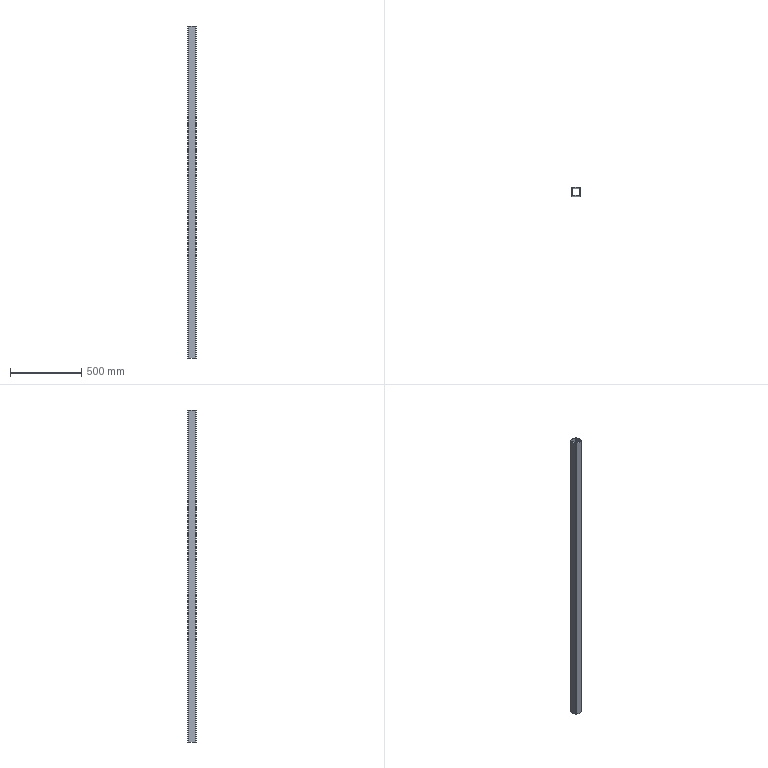Part | STEP file | 750038153 | 1 solid | 18 faces | box 60 x 60 x 2327 mm | volume 2020637 mm3 | plane 10 | cylinder 8 | commonest cylinder face diameters 4 x4 12 x4
STEP:
#1=CARTESIAN_POINT('',(-26.,24.,2326.5));
#2=VERTEX_POINT('',#1);
#3=CARTESIAN_POINT('',(-26.,24.,0.));
#4=VERTEX_POINT('',#3);
#5=CARTESIAN_POINT('',(-26.,24.,2326.5));
#6=DIRECTION('',(0.,0.,-1.));
#7=VECTOR('',#6,1000.);
#8=LINE('',#5,#7);
#9=EDGE_CURVE('',#2,#4,#8,.T.);
#10=ORIENTED_EDGE('',*,*,#9,.F.);
#11=CARTESIAN_POINT('',(-26.,-24.,2326.5));
#12=VERTEX_POINT('',#11);
#13=CARTESIAN_POINT('',(-26.,-24.,2326.5));
#14=DIRECTION('',(0.,1.,0.));
#15=VECTOR('',#14,1000.);
#16=LINE('',#13,#15);
#17=EDGE_CURVE('',#12,#2,#16,.T.);
#18=ORIENTED_EDGE('',*,*,#17,.F.);
#19=CARTESIAN_POINT('',(-26.,-24.,0.));
#20=VERTEX_POINT('',#19);
#21=CARTESIAN_POINT('',(-26.,-24.,2326.5));
#22=DIRECTION('',(0.,0.,1.));
#23=VECTOR('',#22,1000.);
#24=LINE('',#21,#23);
#25=EDGE_CURVE('',#20,#12,#24,.T.);
#26=ORIENTED_EDGE('',*,*,#25,.F.);
#27=CARTESIAN_POINT('',(-26.,-24.,0.));
#28=DIRECTION('',(0.,-1.,0.));
#29=VECTOR('',#28,1000.);
#30=LINE('',#27,#29);
#31=EDGE_CURVE('',#4,#20,#30,.T.);
#32=ORIENTED_EDGE('',*,*,#31,.F.);
#33=EDGE_LOOP('',(#10,#18,#26,#32));
#34=FACE_OUTER_BOUND('',#33,.T.);
#35=CARTESIAN_POINT('',(-26.,-24.,2326.5));
#36=DIRECTION('',(-1.,0.,0.));
#37=DIRECTION('',(0.,-1.,0.));
#38=AXIS2_PLACEMENT_3D('',#35,#36,#37);
#39=PLANE('',#38);
#40=ADVANCED_FACE('',(#34),#39,.F.);
#41=CARTESIAN_POINT('',(26.,24.,0.));
#42=VERTEX_POINT('',#41);
#43=CARTESIAN_POINT('',(24.,26.,0.));
#44=VERTEX_POINT('',#43);
#45=CARTESIAN_POINT('',(24.,24.,0.));
#46=DIRECTION('',(0.,0.,1.));
#47=DIRECTION('',(-1.,0.,0.));
#48=AXIS2_PLACEMENT_3D('',#45,#46,#47);
#49=CIRCLE('',#48,2.);
#50=EDGE_CURVE('',#42,#44,#49,.T.);
#51=ORIENTED_EDGE('',*,*,#50,.T.);
#52=CARTESIAN_POINT('',(-24.,26.,0.));
#53=VERTEX_POINT('',#52);
#54=CARTESIAN_POINT('',(24.,26.,0.));
#55=DIRECTION('',(-1.,0.,0.));
#56=VECTOR('',#55,1000.);
#57=LINE('',#54,#56);
#58=EDGE_CURVE('',#44,#53,#57,.T.);
#59=ORIENTED_EDGE('',*,*,#58,.T.);
#60=CARTESIAN_POINT('',(-24.,24.,0.));
#61=DIRECTION('',(0.,0.,1.));
#62=DIRECTION('',(-1.,0.,0.));
#63=AXIS2_PLACEMENT_3D('',#60,#61,#62);
#64=CIRCLE('',#63,2.);
#65=EDGE_CURVE('',#53,#4,#64,.T.);
#66=ORIENTED_EDGE('',*,*,#65,.T.);
#67=ORIENTED_EDGE('',*,*,#31,.T.);
#68=CARTESIAN_POINT('',(-24.,-26.,0.));
#69=VERTEX_POINT('',#68);
#70=CARTESIAN_POINT('',(-24.,-24.,0.));
#71=DIRECTION('',(0.,0.,1.));
#72=DIRECTION('',(-1.,0.,0.));
#73=AXIS2_PLACEMENT_3D('',#70,#71,#72);
#74=CIRCLE('',#73,2.);
#75=EDGE_CURVE('',#20,#69,#74,.T.);
#76=ORIENTED_EDGE('',*,*,#75,.T.);
#77=CARTESIAN_POINT('',(24.,-26.,0.));
#78=VERTEX_POINT('',#77);
#79=CARTESIAN_POINT('',(24.,-26.,0.));
#80=DIRECTION('',(1.,0.,0.));
#81=VECTOR('',#80,1000.);
#82=LINE('',#79,#81);
#83=EDGE_CURVE('',#69,#78,#82,.T.);
#84=ORIENTED_EDGE('',*,*,#83,.T.);
#85=CARTESIAN_POINT('',(26.,-24.,0.));
#86=VERTEX_POINT('',#85);
#87=CARTESIAN_POINT('',(24.,-24.,0.));
#88=DIRECTION('',(0.,0.,1.));
#89=DIRECTION('',(-1.,0.,0.));
#90=AXIS2_PLACEMENT_3D('',#87,#88,#89);
#91=CIRCLE('',#90,2.);
#92=EDGE_CURVE('',#78,#86,#91,.T.);
#93=ORIENTED_EDGE('',*,*,#92,.T.);
#94=CARTESIAN_POINT('',(26.,-24.,0.));
#95=DIRECTION('',(0.,1.,0.));
#96=VECTOR('',#95,1000.);
#97=LINE('',#94,#96);
#98=EDGE_CURVE('',#86,#42,#97,.T.);
#99=ORIENTED_EDGE('',*,*,#98,.T.);
#100=EDGE_LOOP('',(#51,#59,#66,#67,#76,#84,#93,#99));
#101=FACE_BOUND('',#100,.T.);
#102=CARTESIAN_POINT('',(-24.,30.,0.));
#103=VERTEX_POINT('',#102);
#104=CARTESIAN_POINT('',(24.,30.,0.));
#105=VERTEX_POINT('',#104);
#106=CARTESIAN_POINT('',(24.,30.,0.));
#107=DIRECTION('',(1.,0.,0.));
#108=VECTOR('',#107,1000.);
#109=LINE('',#106,#108);
#110=EDGE_CURVE('',#103,#105,#109,.T.);
#111=ORIENTED_EDGE('',*,*,#110,.T.);
#112=CARTESIAN_POINT('',(30.,24.,0.));
#113=VERTEX_POINT('',#112);
#114=CARTESIAN_POINT('',(24.,24.,0.));
#115=DIRECTION('',(0.,0.,-1.));
#116=DIRECTION('',(-1.,0.,0.));
#117=AXIS2_PLACEMENT_3D('',#114,#115,#116);
#118=CIRCLE('',#117,6.);
#119=EDGE_CURVE('',#105,#113,#118,.T.);
#120=ORIENTED_EDGE('',*,*,#119,.T.);
#121=CARTESIAN_POINT('',(30.,-24.,0.));
#122=VERTEX_POINT('',#121);
#123=CARTESIAN_POINT('',(30.,-24.,0.));
#124=DIRECTION('',(0.,-1.,0.));
#125=VECTOR('',#124,1000.);
#126=LINE('',#123,#125);
#127=EDGE_CURVE('',#113,#122,#126,.T.);
#128=ORIENTED_EDGE('',*,*,#127,.T.);
#129=CARTESIAN_POINT('',(24.,-30.,0.));
#130=VERTEX_POINT('',#129);
#131=CARTESIAN_POINT('',(24.,-24.,0.));
#132=DIRECTION('',(0.,0.,-1.));
#133=DIRECTION('',(-1.,0.,0.));
#134=AXIS2_PLACEMENT_3D('',#131,#132,#133);
#135=CIRCLE('',#134,6.);
#136=EDGE_CURVE('',#122,#130,#135,.T.);
#137=ORIENTED_EDGE('',*,*,#136,.T.);
#138=CARTESIAN_POINT('',(-24.,-30.,0.));
#139=VERTEX_POINT('',#138);
#140=CARTESIAN_POINT('',(24.,-30.,0.));
#141=DIRECTION('',(-1.,0.,0.));
#142=VECTOR('',#141,1000.);
#143=LINE('',#140,#142);
#144=EDGE_CURVE('',#130,#139,#143,.T.);
#145=ORIENTED_EDGE('',*,*,#144,.T.);
#146=CARTESIAN_POINT('',(-30.,-24.,0.));
#147=VERTEX_POINT('',#146);
#148=CARTESIAN_POINT('',(-24.,-24.,0.));
#149=DIRECTION('',(0.,0.,-1.));
#150=DIRECTION('',(-1.,0.,0.));
#151=AXIS2_PLACEMENT_3D('',#148,#149,#150);
#152=CIRCLE('',#151,6.);
#153=EDGE_CURVE('',#139,#147,#152,.T.);
#154=ORIENTED_EDGE('',*,*,#153,.T.);
#155=CARTESIAN_POINT('',(-30.,24.,0.));
#156=VERTEX_POINT('',#155);
#157=CARTESIAN_POINT('',(-30.,-24.,0.));
#158=DIRECTION('',(0.,1.,0.));
#159=VECTOR('',#158,1000.);
#160=LINE('',#157,#159);
#161=EDGE_CURVE('',#147,#156,#160,.T.);
#162=ORIENTED_EDGE('',*,*,#161,.T.);
#163=CARTESIAN_POINT('',(-24.,24.,0.));
#164=DIRECTION('',(0.,0.,-1.));
#165=DIRECTION('',(-1.,0.,0.));
#166=AXIS2_PLACEMENT_3D('',#163,#164,#165);
#167=CIRCLE('',#166,6.);
#168=EDGE_CURVE('',#156,#103,#167,.T.);
#169=ORIENTED_EDGE('',*,*,#168,.T.);
#170=EDGE_LOOP('',(#111,#120,#128,#137,#145,#154,#162,#169));
#171=FACE_OUTER_BOUND('',#170,.T.);
#172=CARTESIAN_POINT('',(24.,-24.,0.));
#173=DIRECTION('',(0.,0.,-1.));
#174=DIRECTION('',(-1.,0.,0.));
#175=AXIS2_PLACEMENT_3D('',#172,#173,#174);
#176=PLANE('',#175);
#177=ADVANCED_FACE('',(#101,#171),#176,.T.);
#178=CARTESIAN_POINT('',(-24.,26.,2326.5));
#179=VERTEX_POINT('',#178);
#180=CARTESIAN_POINT('',(-24.,26.,2326.5));
#181=DIRECTION('',(0.,0.,-1.));
#182=VECTOR('',#181,1000.);
#183=LINE('',#180,#182);
#184=EDGE_CURVE('',#179,#53,#183,.T.);
#185=ORIENTED_EDGE('',*,*,#184,.F.);
#186=CARTESIAN_POINT('',(-24.,24.,2326.5));
#187=DIRECTION('',(0.,0.,-1.));
#188=DIRECTION('',(-1.,0.,0.));
#189=AXIS2_PLACEMENT_3D('',#186,#187,#188);
#190=CIRCLE('',#189,2.);
#191=EDGE_CURVE('',#2,#179,#190,.T.);
#192=ORIENTED_EDGE('',*,*,#191,.F.);
#193=ORIENTED_EDGE('',*,*,#9,.T.);
#194=ORIENTED_EDGE('',*,*,#65,.F.);
#195=EDGE_LOOP('',(#185,#192,#193,#194));
#196=FACE_OUTER_BOUND('',#195,.T.);
#197=CARTESIAN_POINT('',(-24.,24.,2326.5));
#198=DIRECTION('',(0.,0.,-1.));
#199=DIRECTION('',(-1.,0.,0.));
#200=AXIS2_PLACEMENT_3D('',#197,#198,#199);
#201=CYLINDRICAL_SURFACE('',#200,2.);
#202=ADVANCED_FACE('',(#196),#201,.F.);
#203=CARTESIAN_POINT('',(24.,26.,2326.5));
#204=VERTEX_POINT('',#203);
#205=CARTESIAN_POINT('',(24.,26.,2326.5));
#206=DIRECTION('',(-1.,0.,0.));
#207=VECTOR('',#206,1000.);
#208=LINE('',#205,#207);
#209=EDGE_CURVE('',#204,#179,#208,.T.);
#210=ORIENTED_EDGE('',*,*,#209,.F.);
#211=CARTESIAN_POINT('',(26.,24.,2326.5));
#212=VERTEX_POINT('',#211);
#213=CARTESIAN_POINT('',(24.,24.,2326.5));
#214=DIRECTION('',(0.,0.,1.));
#215=DIRECTION('',(-1.,0.,0.));
#216=AXIS2_PLACEMENT_3D('',#213,#214,#215);
#217=CIRCLE('',#216,2.);
#218=EDGE_CURVE('',#212,#204,#217,.T.);
#219=ORIENTED_EDGE('',*,*,#218,.F.);
#220=CARTESIAN_POINT('',(26.,-24.,2326.5));
#221=VERTEX_POINT('',#220);
#222=CARTESIAN_POINT('',(26.,-24.,2326.5));
#223=DIRECTION('',(0.,1.,0.));
#224=VECTOR('',#223,1000.);
#225=LINE('',#222,#224);
#226=EDGE_CURVE('',#221,#212,#225,.T.);
#227=ORIENTED_EDGE('',*,*,#226,.F.);
#228=CARTESIAN_POINT('',(24.,-26.,2326.5));
#229=VERTEX_POINT('',#228);
#230=CARTESIAN_POINT('',(24.,-24.,2326.5));
#231=DIRECTION('',(0.,0.,1.));
#232=DIRECTION('',(-1.,0.,0.));
#233=AXIS2_PLACEMENT_3D('',#230,#231,#232);
#234=CIRCLE('',#233,2.);
#235=EDGE_CURVE('',#229,#221,#234,.T.);
#236=ORIENTED_EDGE('',*,*,#235,.F.);
#237=CARTESIAN_POINT('',(-24.,-26.,2326.5));
#238=VERTEX_POINT('',#237);
#239=CARTESIAN_POINT('',(24.,-26.,2326.5));
#240=DIRECTION('',(1.,0.,0.));
#241=VECTOR('',#240,1000.);
#242=LINE('',#239,#241);
#243=EDGE_CURVE('',#238,#229,#242,.T.);
#244=ORIENTED_EDGE('',*,*,#243,.F.);
#245=CARTESIAN_POINT('',(-24.,-24.,2326.5));
#246=DIRECTION('',(0.,0.,1.));
#247=DIRECTION('',(-1.,0.,0.));
#248=AXIS2_PLACEMENT_3D('',#245,#246,#247);
#249=CIRCLE('',#248,2.);
#250=EDGE_CURVE('',#12,#238,#249,.T.);
#251=ORIENTED_EDGE('',*,*,#250,.F.);
#252=ORIENTED_EDGE('',*,*,#17,.T.);
#253=ORIENTED_EDGE('',*,*,#191,.T.);
#254=EDGE_LOOP('',(#210,#219,#227,#236,#244,#251,#252,#253));
#255=FACE_BOUND('',#254,.T.);
#256=CARTESIAN_POINT('',(24.,30.,2326.5));
#257=VERTEX_POINT('',#256);
#258=CARTESIAN_POINT('',(30.,24.,2326.5));
#259=VERTEX_POINT('',#258);
#260=CARTESIAN_POINT('',(24.,24.,2326.5));
#261=DIRECTION('',(0.,0.,-1.));
#262=DIRECTION('',(-1.,0.,0.));
#263=AXIS2_PLACEMENT_3D('',#260,#261,#262);
#264=CIRCLE('',#263,6.);
#265=EDGE_CURVE('',#257,#259,#264,.T.);
#266=ORIENTED_EDGE('',*,*,#265,.F.);
#267=CARTESIAN_POINT('',(-24.,30.,2326.5));
#268=VERTEX_POINT('',#267);
#269=CARTESIAN_POINT('',(24.,30.,2326.5));
#270=DIRECTION('',(1.,0.,0.));
#271=VECTOR('',#270,1000.);
#272=LINE('',#269,#271);
#273=EDGE_CURVE('',#268,#257,#272,.T.);
#274=ORIENTED_EDGE('',*,*,#273,.F.);
#275=CARTESIAN_POINT('',(-30.,24.,2326.5));
#276=VERTEX_POINT('',#275);
#277=CARTESIAN_POINT('',(-24.,24.,2326.5));
#278=DIRECTION('',(0.,0.,-1.));
#279=DIRECTION('',(-1.,0.,0.));
#280=AXIS2_PLACEMENT_3D('',#277,#278,#279);
#281=CIRCLE('',#280,6.);
#282=EDGE_CURVE('',#276,#268,#281,.T.);
#283=ORIENTED_EDGE('',*,*,#282,.F.);
#284=CARTESIAN_POINT('',(-30.,-24.,2326.5));
#285=VERTEX_POINT('',#284);
#286=CARTESIAN_POINT('',(-30.,-24.,2326.5));
#287=DIRECTION('',(0.,1.,0.));
#288=VECTOR('',#287,1000.);
#289=LINE('',#286,#288);
#290=EDGE_CURVE('',#285,#276,#289,.T.);
#291=ORIENTED_EDGE('',*,*,#290,.F.);
#292=CARTESIAN_POINT('',(-24.,-30.,2326.5));
#293=VERTEX_POINT('',#292);
#294=CARTESIAN_POINT('',(-24.,-24.,2326.5));
#295=DIRECTION('',(0.,0.,-1.));
#296=DIRECTION('',(-1.,0.,0.));
#297=AXIS2_PLACEMENT_3D('',#294,#295,#296);
#298=CIRCLE('',#297,6.);
#299=EDGE_CURVE('',#293,#285,#298,.T.);
#300=ORIENTED_EDGE('',*,*,#299,.F.);
#301=CARTESIAN_POINT('',(24.,-30.,2326.5));
#302=VERTEX_POINT('',#301);
#303=CARTESIAN_POINT('',(24.,-30.,2326.5));
#304=DIRECTION('',(-1.,0.,0.));
#305=VECTOR('',#304,1000.);
#306=LINE('',#303,#305);
#307=EDGE_CURVE('',#302,#293,#306,.T.);
#308=ORIENTED_EDGE('',*,*,#307,.F.);
#309=CARTESIAN_POINT('',(30.,-24.,2326.5));
#310=VERTEX_POINT('',#309);
#311=CARTESIAN_POINT('',(24.,-24.,2326.5));
#312=DIRECTION('',(0.,0.,-1.));
#313=DIRECTION('',(-1.,0.,0.));
#314=AXIS2_PLACEMENT_3D('',#311,#312,#313);
#315=CIRCLE('',#314,6.);
#316=EDGE_CURVE('',#310,#302,#315,.T.);
#317=ORIENTED_EDGE('',*,*,#316,.F.);
#318=CARTESIAN_POINT('',(30.,-24.,2326.5));
#319=DIRECTION('',(0.,-1.,0.));
#320=VECTOR('',#319,1000.);
#321=LINE('',#318,#320);
#322=EDGE_CURVE('',#259,#310,#321,.T.);
#323=ORIENTED_EDGE('',*,*,#322,.F.);
#324=EDGE_LOOP('',(#266,#274,#283,#291,#300,#308,#317,#323));
#325=FACE_OUTER_BOUND('',#324,.T.);
#326=CARTESIAN_POINT('',(24.,-24.,2326.5));
#327=DIRECTION('',(0.,0.,-1.));
#328=DIRECTION('',(-1.,0.,0.));
#329=AXIS2_PLACEMENT_3D('',#326,#327,#328);
#330=PLANE('',#329);
#331=ADVANCED_FACE('',(#255,#325),#330,.F.);
#332=ORIENTED_EDGE('',*,*,#25,.T.);
#333=ORIENTED_EDGE('',*,*,#250,.T.);
#334=CARTESIAN_POINT('',(-24.,-26.,2326.5));
#335=DIRECTION('',(0.,0.,1.));
#336=VECTOR('',#335,1000.);
#337=LINE('',#334,#336);
#338=EDGE_CURVE('',#69,#238,#337,.T.);
#339=ORIENTED_EDGE('',*,*,#338,.F.);
#340=ORIENTED_EDGE('',*,*,#75,.F.);
#341=EDGE_LOOP('',(#332,#333,#339,#340));
#342=FACE_OUTER_BOUND('',#341,.T.);
#343=CARTESIAN_POINT('',(-24.,-24.,2326.5));
#344=DIRECTION('',(0.,0.,-1.));
#345=DIRECTION('',(-1.,0.,0.));
#346=AXIS2_PLACEMENT_3D('',#343,#344,#345);
#347=CYLINDRICAL_SURFACE('',#346,2.);
#348=ADVANCED_FACE('',(#342),#347,.F.);
#349=CARTESIAN_POINT('',(24.,26.,2326.5));
#350=DIRECTION('',(0.,0.,-1.));
#351=VECTOR('',#350,1000.);
#352=LINE('',#349,#351);
#353=EDGE_CURVE('',#204,#44,#352,.T.);
#354=ORIENTED_EDGE('',*,*,#353,.F.);
#355=ORIENTED_EDGE('',*,*,#209,.T.);
#356=ORIENTED_EDGE('',*,*,#184,.T.);
#357=ORIENTED_EDGE('',*,*,#58,.F.);
#358=EDGE_LOOP('',(#354,#355,#356,#357));
#359=FACE_OUTER_BOUND('',#358,.T.);
#360=CARTESIAN_POINT('',(-24.,26.,2326.5));
#361=DIRECTION('',(0.,1.,0.));
#362=DIRECTION('',(0.,0.,1.));
#363=AXIS2_PLACEMENT_3D('',#360,#361,#362);
#364=PLANE('',#363);
#365=ADVANCED_FACE('',(#359),#364,.F.);
#366=CARTESIAN_POINT('',(26.,24.,2326.5));
#367=DIRECTION('',(0.,0.,-1.));
#368=VECTOR('',#367,1000.);
#369=LINE('',#366,#368);
#370=EDGE_CURVE('',#212,#42,#369,.T.);
#371=ORIENTED_EDGE('',*,*,#370,.F.);
#372=ORIENTED_EDGE('',*,*,#218,.T.);
#373=ORIENTED_EDGE('',*,*,#353,.T.);
#374=ORIENTED_EDGE('',*,*,#50,.F.);
#375=EDGE_LOOP('',(#371,#372,#373,#374));
#376=FACE_OUTER_BOUND('',#375,.T.);
#377=CARTESIAN_POINT('',(24.,24.,2326.5));
#378=DIRECTION('',(0.,0.,-1.));
#379=DIRECTION('',(-1.,0.,0.));
#380=AXIS2_PLACEMENT_3D('',#377,#378,#379);
#381=CYLINDRICAL_SURFACE('',#380,2.);
#382=ADVANCED_FACE('',(#376),#381,.F.);
#383=CARTESIAN_POINT('',(26.,-24.,2326.5));
#384=DIRECTION('',(0.,0.,-1.));
#385=VECTOR('',#384,1000.);
#386=LINE('',#383,#385);
#387=EDGE_CURVE('',#221,#86,#386,.T.);
#388=ORIENTED_EDGE('',*,*,#387,.F.);
#389=ORIENTED_EDGE('',*,*,#226,.T.);
#390=ORIENTED_EDGE('',*,*,#370,.T.);
#391=ORIENTED_EDGE('',*,*,#98,.F.);
#392=EDGE_LOOP('',(#388,#389,#390,#391));
#393=FACE_OUTER_BOUND('',#392,.T.);
#394=CARTESIAN_POINT('',(26.,24.,2326.5));
#395=DIRECTION('',(1.,0.,0.));
#396=DIRECTION('',(0.,0.,-1.));
#397=AXIS2_PLACEMENT_3D('',#394,#395,#396);
#398=PLANE('',#397);
#399=ADVANCED_FACE('',(#393),#398,.F.);
#400=CARTESIAN_POINT('',(24.,-26.,2326.5));
#401=DIRECTION('',(0.,0.,-1.));
#402=VECTOR('',#401,1000.);
#403=LINE('',#400,#402);
#404=EDGE_CURVE('',#229,#78,#403,.T.);
#405=ORIENTED_EDGE('',*,*,#404,.F.);
#406=ORIENTED_EDGE('',*,*,#235,.T.);
#407=ORIENTED_EDGE('',*,*,#387,.T.);
#408=ORIENTED_EDGE('',*,*,#92,.F.);
#409=EDGE_LOOP('',(#405,#406,#407,#408));
#410=FACE_OUTER_BOUND('',#409,.T.);
#411=CARTESIAN_POINT('',(24.,-24.,2326.5));
#412=DIRECTION('',(0.,0.,-1.));
#413=DIRECTION('',(-1.,0.,0.));
#414=AXIS2_PLACEMENT_3D('',#411,#412,#413);
#415=CYLINDRICAL_SURFACE('',#414,2.);
#416=ADVANCED_FACE('',(#410),#415,.F.);
#417=ORIENTED_EDGE('',*,*,#338,.T.);
#418=ORIENTED_EDGE('',*,*,#243,.T.);
#419=ORIENTED_EDGE('',*,*,#404,.T.);
#420=ORIENTED_EDGE('',*,*,#83,.F.);
#421=EDGE_LOOP('',(#417,#418,#419,#420));
#422=FACE_OUTER_BOUND('',#421,.T.);
#423=CARTESIAN_POINT('',(24.,-26.,2326.5));
#424=DIRECTION('',(0.,-1.,0.));
#425=DIRECTION('',(0.,0.,-1.));
#426=AXIS2_PLACEMENT_3D('',#423,#424,#425);
#427=PLANE('',#426);
#428=ADVANCED_FACE('',(#422),#427,.F.);
#429=ORIENTED_EDGE('',*,*,#265,.T.);
#430=CARTESIAN_POINT('',(30.,24.,2326.5));
#431=DIRECTION('',(0.,0.,-1.));
#432=VECTOR('',#431,1000.);
#433=LINE('',#430,#432);
#434=EDGE_CURVE('',#259,#113,#433,.T.);
#435=ORIENTED_EDGE('',*,*,#434,.T.);
#436=ORIENTED_EDGE('',*,*,#119,.F.);
#437=CARTESIAN_POINT('',(24.,30.,2326.5));
#438=DIRECTION('',(0.,0.,1.));
#439=VECTOR('',#438,1000.);
#440=LINE('',#437,#439);
#441=EDGE_CURVE('',#105,#257,#440,.T.);
#442=ORIENTED_EDGE('',*,*,#441,.T.);
#443=EDGE_LOOP('',(#429,#435,#436,#442));
#444=FACE_OUTER_BOUND('',#443,.T.);
#445=CARTESIAN_POINT('',(24.,24.,2326.5));
#446=DIRECTION('',(0.,0.,-1.));
#447=DIRECTION('',(-1.,0.,0.));
#448=AXIS2_PLACEMENT_3D('',#445,#446,#447);
#449=CYLINDRICAL_SURFACE('',#448,6.);
#450=ADVANCED_FACE('',(#444),#449,.T.);
#451=ORIENTED_EDGE('',*,*,#273,.T.);
#452=ORIENTED_EDGE('',*,*,#441,.F.);
#453=ORIENTED_EDGE('',*,*,#110,.F.);
#454=CARTESIAN_POINT('',(-24.,30.,2326.5));
#455=DIRECTION('',(0.,0.,1.));
#456=VECTOR('',#455,1000.);
#457=LINE('',#454,#456);
#458=EDGE_CURVE('',#103,#268,#457,.T.);
#459=ORIENTED_EDGE('',*,*,#458,.T.);
#460=EDGE_LOOP('',(#451,#452,#453,#459));
#461=FACE_OUTER_BOUND('',#460,.T.);
#462=CARTESIAN_POINT('',(-24.,30.,2326.5));
#463=DIRECTION('',(0.,1.,0.));
#464=DIRECTION('',(-1.,0.,0.));
#465=AXIS2_PLACEMENT_3D('',#462,#463,#464);
#466=PLANE('',#465);
#467=ADVANCED_FACE('',(#461),#466,.T.);
#468=ORIENTED_EDGE('',*,*,#282,.T.);
#469=ORIENTED_EDGE('',*,*,#458,.F.);
#470=ORIENTED_EDGE('',*,*,#168,.F.);
#471=CARTESIAN_POINT('',(-30.,24.,2326.5));
#472=DIRECTION('',(0.,0.,1.));
#473=VECTOR('',#472,1000.);
#474=LINE('',#471,#473);
#475=EDGE_CURVE('',#156,#276,#474,.T.);
#476=ORIENTED_EDGE('',*,*,#475,.T.);
#477=EDGE_LOOP('',(#468,#469,#470,#476));
#478=FACE_OUTER_BOUND('',#477,.T.);
#479=CARTESIAN_POINT('',(-24.,24.,2326.5));
#480=DIRECTION('',(0.,0.,-1.));
#481=DIRECTION('',(-1.,0.,0.));
#482=AXIS2_PLACEMENT_3D('',#479,#480,#481);
#483=CYLINDRICAL_SURFACE('',#482,6.);
#484=ADVANCED_FACE('',(#478),#483,.T.);
#485=ORIENTED_EDGE('',*,*,#290,.T.);
#486=ORIENTED_EDGE('',*,*,#475,.F.);
#487=ORIENTED_EDGE('',*,*,#161,.F.);
#488=CARTESIAN_POINT('',(-30.,-24.,2326.5));
#489=DIRECTION('',(0.,0.,1.));
#490=VECTOR('',#489,1000.);
#491=LINE('',#488,#490);
#492=EDGE_CURVE('',#147,#285,#491,.T.);
#493=ORIENTED_EDGE('',*,*,#492,.T.);
#494=EDGE_LOOP('',(#485,#486,#487,#493));
#495=FACE_OUTER_BOUND('',#494,.T.);
#496=CARTESIAN_POINT('',(-30.,-24.,2326.5));
#497=DIRECTION('',(-1.,0.,0.));
#498=DIRECTION('',(0.,-1.,0.));
#499=AXIS2_PLACEMENT_3D('',#496,#497,#498);
#500=PLANE('',#499);
#501=ADVANCED_FACE('',(#495),#500,.T.);
#502=ORIENTED_EDGE('',*,*,#299,.T.);
#503=ORIENTED_EDGE('',*,*,#492,.F.);
#504=ORIENTED_EDGE('',*,*,#153,.F.);
#505=CARTESIAN_POINT('',(-24.,-30.,2326.5));
#506=DIRECTION('',(0.,0.,1.));
#507=VECTOR('',#506,1000.);
#508=LINE('',#505,#507);
#509=EDGE_CURVE('',#139,#293,#508,.T.);
#510=ORIENTED_EDGE('',*,*,#509,.T.);
#511=EDGE_LOOP('',(#502,#503,#504,#510));
#512=FACE_OUTER_BOUND('',#511,.T.);
#513=CARTESIAN_POINT('',(-24.,-24.,2326.5));
#514=DIRECTION('',(0.,0.,-1.));
#515=DIRECTION('',(-1.,0.,0.));
#516=AXIS2_PLACEMENT_3D('',#513,#514,#515);
#517=CYLINDRICAL_SURFACE('',#516,6.);
#518=ADVANCED_FACE('',(#512),#517,.T.);
#519=ORIENTED_EDGE('',*,*,#307,.T.);
#520=ORIENTED_EDGE('',*,*,#509,.F.);
#521=ORIENTED_EDGE('',*,*,#144,.F.);
#522=CARTESIAN_POINT('',(24.,-30.,2326.5));
#523=DIRECTION('',(0.,0.,1.));
#524=VECTOR('',#523,1000.);
#525=LINE('',#522,#524);
#526=EDGE_CURVE('',#130,#302,#525,.T.);
#527=ORIENTED_EDGE('',*,*,#526,.T.);
#528=EDGE_LOOP('',(#519,#520,#521,#527));
#529=FACE_OUTER_BOUND('',#528,.T.);
#530=CARTESIAN_POINT('',(24.,-30.,2326.5));
#531=DIRECTION('',(0.,-1.,0.));
#532=DIRECTION('',(1.,0.,0.));
#533=AXIS2_PLACEMENT_3D('',#530,#531,#532);
#534=PLANE('',#533);
#535=ADVANCED_FACE('',(#529),#534,.T.);
#536=ORIENTED_EDGE('',*,*,#316,.T.);
#537=ORIENTED_EDGE('',*,*,#526,.F.);
#538=ORIENTED_EDGE('',*,*,#136,.F.);
#539=CARTESIAN_POINT('',(30.,-24.,2326.5));
#540=DIRECTION('',(0.,0.,1.));
#541=VECTOR('',#540,1000.);
#542=LINE('',#539,#541);
#543=EDGE_CURVE('',#122,#310,#542,.T.);
#544=ORIENTED_EDGE('',*,*,#543,.T.);
#545=EDGE_LOOP('',(#536,#537,#538,#544));
#546=FACE_OUTER_BOUND('',#545,.T.);
#547=CARTESIAN_POINT('',(24.,-24.,2326.5));
#548=DIRECTION('',(0.,0.,-1.));
#549=DIRECTION('',(-1.,0.,0.));
#550=AXIS2_PLACEMENT_3D('',#547,#548,#549);
#551=CYLINDRICAL_SURFACE('',#550,6.);
#552=ADVANCED_FACE('',(#546),#551,.T.);
#553=ORIENTED_EDGE('',*,*,#322,.T.);
#554=ORIENTED_EDGE('',*,*,#543,.F.);
#555=ORIENTED_EDGE('',*,*,#127,.F.);
#556=ORIENTED_EDGE('',*,*,#434,.F.);
#557=EDGE_LOOP('',(#553,#554,#555,#556));
#558=FACE_OUTER_BOUND('',#557,.T.);
#559=CARTESIAN_POINT('',(30.,24.,2326.5));
#560=DIRECTION('',(1.,0.,0.));
#561=DIRECTION('',(0.,0.,-1.));
#562=AXIS2_PLACEMENT_3D('',#559,#560,#561);
#563=PLANE('',#562);
#564=ADVANCED_FACE('',(#558),#563,.T.);
#565=CLOSED_SHELL('',(#40,#177,#202,#331,#348,#365,#382,#399,#416,#428,#450,#467,#484,#501,#518,#535,#552,#564));
#566=MANIFOLD_SOLID_BREP('',#565);
#567=CARTESIAN_POINT('',(0.,0.,0.));
#568=DIRECTION('',(0.,0.,1.));
#569=DIRECTION('',(1.,0.,0.));
#570=AXIS2_PLACEMENT_3D('',#567,#568,#569);
#571=(LENGTH_UNIT()NAMED_UNIT(*)SI_UNIT(.MILLI.,.METRE.));
#572=UNCERTAINTY_MEASURE_WITH_UNIT(LENGTH_MEASURE(0.00001),#571,'','');
#573=(NAMED_UNIT(*)PLANE_ANGLE_UNIT()SI_UNIT($,.RADIAN.));
#574=(NAMED_UNIT(*)SI_UNIT($,.STERADIAN.)SOLID_ANGLE_UNIT());
#575=(GEOMETRIC_REPRESENTATION_CONTEXT(3)GLOBAL_UNCERTAINTY_ASSIGNED_CONTEXT((#572))GLOBAL_UNIT_ASSIGNED_CONTEXT((#571,#573,#574))REPRESENTATION_CONTEXT('',''));
#576=ADVANCED_BREP_SHAPE_REPRESENTATION('',(#566,#570),#575);